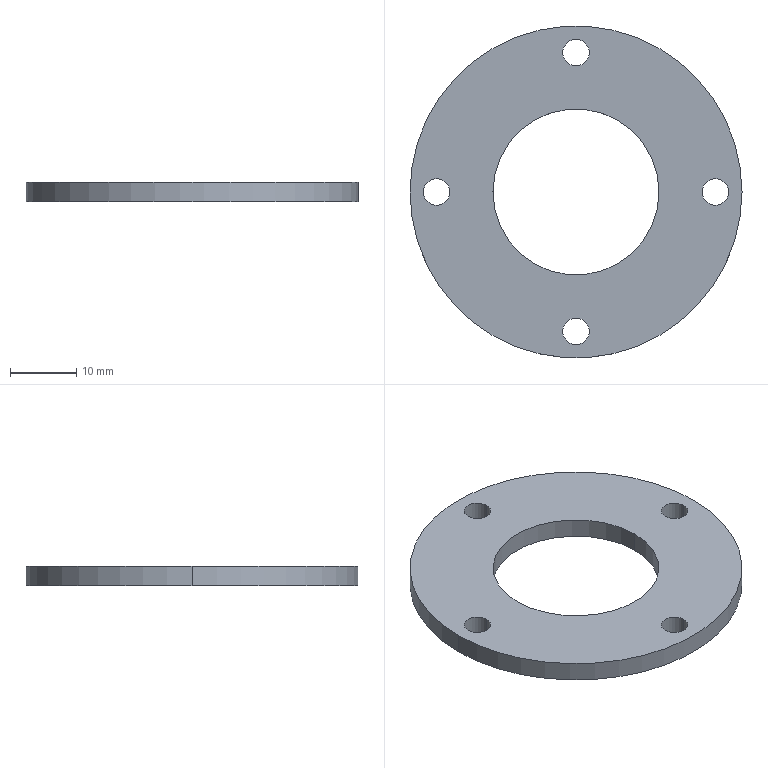Part | SolidWorks | features BaseBody 1 | 1 solid | 14 faces | box 50 x 50 x 3 mm | volume 4267 mm3 | cylinder 12 | plane 2 | commonest cylinder face diameters 4 x8 25 x2 50 x2
STEP:
#1=CARTESIAN_POINT('',(12.5,0.,0.));
#2=VERTEX_POINT('',#1);
#3=CARTESIAN_POINT('',(-12.5,0.,0.));
#4=VERTEX_POINT('',#3);
#5=CARTESIAN_POINT('',(0.,0.,0.));
#6=DIRECTION('',(0.,0.,-1.));
#7=DIRECTION('',(1.,0.,0.));
#8=AXIS2_PLACEMENT_3D('',#5,#6,#7);
#9=CIRCLE('',#8,12.5);
#10=EDGE_CURVE('',#2,#4,#9,.T.);
#11=ORIENTED_EDGE('',*,*,#10,.T.);
#12=CARTESIAN_POINT('',(-12.5,0.,3.));
#13=VERTEX_POINT('',#12);
#14=CARTESIAN_POINT('',(-12.5,0.,0.));
#15=DIRECTION('',(0.,0.,1.));
#16=VECTOR('',#15,1000.);
#17=LINE('',#14,#16);
#18=EDGE_CURVE('',#4,#13,#17,.T.);
#19=ORIENTED_EDGE('',*,*,#18,.T.);
#20=CARTESIAN_POINT('',(12.5,0.,3.));
#21=VERTEX_POINT('',#20);
#22=CARTESIAN_POINT('',(0.,0.,3.));
#23=DIRECTION('',(0.,0.,1.));
#24=DIRECTION('',(1.,0.,0.));
#25=AXIS2_PLACEMENT_3D('',#22,#23,#24);
#26=CIRCLE('',#25,12.5);
#27=EDGE_CURVE('',#13,#21,#26,.T.);
#28=ORIENTED_EDGE('',*,*,#27,.T.);
#29=CARTESIAN_POINT('',(12.5,0.,0.));
#30=DIRECTION('',(0.,0.,1.));
#31=VECTOR('',#30,1000.);
#32=LINE('',#29,#31);
#33=EDGE_CURVE('',#2,#21,#32,.T.);
#34=ORIENTED_EDGE('',*,*,#33,.F.);
#35=EDGE_LOOP('',(#11,#19,#28,#34));
#36=FACE_OUTER_BOUND('',#35,.T.);
#37=CARTESIAN_POINT('',(0.,0.,0.));
#38=DIRECTION('',(0.,0.,1.));
#39=DIRECTION('',(1.,0.,0.));
#40=AXIS2_PLACEMENT_3D('',#37,#38,#39);
#41=CYLINDRICAL_SURFACE('',#40,12.5);
#42=ADVANCED_FACE('',(#36),#41,.F.);
#43=CARTESIAN_POINT('',(2.,21.,0.));
#44=VERTEX_POINT('',#43);
#45=CARTESIAN_POINT('',(-2.,21.,0.));
#46=VERTEX_POINT('',#45);
#47=CARTESIAN_POINT('',(0.,21.,0.));
#48=DIRECTION('',(0.,0.,-1.));
#49=DIRECTION('',(1.,0.,0.));
#50=AXIS2_PLACEMENT_3D('',#47,#48,#49);
#51=CIRCLE('',#50,2.);
#52=EDGE_CURVE('',#44,#46,#51,.T.);
#53=ORIENTED_EDGE('',*,*,#52,.T.);
#54=CARTESIAN_POINT('',(-2.,21.,3.));
#55=VERTEX_POINT('',#54);
#56=CARTESIAN_POINT('',(-2.,21.,0.));
#57=DIRECTION('',(0.,0.,1.));
#58=VECTOR('',#57,1000.);
#59=LINE('',#56,#58);
#60=EDGE_CURVE('',#46,#55,#59,.T.);
#61=ORIENTED_EDGE('',*,*,#60,.T.);
#62=CARTESIAN_POINT('',(2.,21.,3.));
#63=VERTEX_POINT('',#62);
#64=CARTESIAN_POINT('',(0.,21.,3.));
#65=DIRECTION('',(0.,0.,-1.));
#66=DIRECTION('',(1.,0.,0.));
#67=AXIS2_PLACEMENT_3D('',#64,#65,#66);
#68=CIRCLE('',#67,2.);
#69=EDGE_CURVE('',#63,#55,#68,.T.);
#70=ORIENTED_EDGE('',*,*,#69,.F.);
#71=CARTESIAN_POINT('',(2.,21.,0.));
#72=DIRECTION('',(0.,0.,1.));
#73=VECTOR('',#72,1000.);
#74=LINE('',#71,#73);
#75=EDGE_CURVE('',#44,#63,#74,.T.);
#76=ORIENTED_EDGE('',*,*,#75,.F.);
#77=EDGE_LOOP('',(#53,#61,#70,#76));
#78=FACE_OUTER_BOUND('',#77,.T.);
#79=CARTESIAN_POINT('',(0.,21.,0.));
#80=DIRECTION('',(0.,0.,1.));
#81=DIRECTION('',(1.,0.,0.));
#82=AXIS2_PLACEMENT_3D('',#79,#80,#81);
#83=CYLINDRICAL_SURFACE('',#82,2.);
#84=ADVANCED_FACE('',(#78),#83,.F.);
#85=CARTESIAN_POINT('',(23.,0.,0.));
#86=VERTEX_POINT('',#85);
#87=CARTESIAN_POINT('',(19.,0.,0.));
#88=VERTEX_POINT('',#87);
#89=CARTESIAN_POINT('',(21.,0.,0.));
#90=DIRECTION('',(0.,0.,-1.));
#91=DIRECTION('',(1.,0.,0.));
#92=AXIS2_PLACEMENT_3D('',#89,#90,#91);
#93=CIRCLE('',#92,2.);
#94=EDGE_CURVE('',#86,#88,#93,.T.);
#95=ORIENTED_EDGE('',*,*,#94,.T.);
#96=CARTESIAN_POINT('',(19.,0.,3.));
#97=VERTEX_POINT('',#96);
#98=CARTESIAN_POINT('',(19.,0.,0.));
#99=DIRECTION('',(0.,0.,1.));
#100=VECTOR('',#99,1000.);
#101=LINE('',#98,#100);
#102=EDGE_CURVE('',#88,#97,#101,.T.);
#103=ORIENTED_EDGE('',*,*,#102,.T.);
#104=CARTESIAN_POINT('',(23.,0.,3.));
#105=VERTEX_POINT('',#104);
#106=CARTESIAN_POINT('',(21.,0.,3.));
#107=DIRECTION('',(0.,0.,-1.));
#108=DIRECTION('',(1.,0.,0.));
#109=AXIS2_PLACEMENT_3D('',#106,#107,#108);
#110=CIRCLE('',#109,2.);
#111=EDGE_CURVE('',#105,#97,#110,.T.);
#112=ORIENTED_EDGE('',*,*,#111,.F.);
#113=CARTESIAN_POINT('',(23.,0.,0.));
#114=DIRECTION('',(0.,0.,1.));
#115=VECTOR('',#114,1000.);
#116=LINE('',#113,#115);
#117=EDGE_CURVE('',#86,#105,#116,.T.);
#118=ORIENTED_EDGE('',*,*,#117,.F.);
#119=EDGE_LOOP('',(#95,#103,#112,#118));
#120=FACE_OUTER_BOUND('',#119,.T.);
#121=CARTESIAN_POINT('',(21.,0.,0.));
#122=DIRECTION('',(0.,0.,1.));
#123=DIRECTION('',(1.,0.,0.));
#124=AXIS2_PLACEMENT_3D('',#121,#122,#123);
#125=CYLINDRICAL_SURFACE('',#124,2.);
#126=ADVANCED_FACE('',(#120),#125,.F.);
#127=CARTESIAN_POINT('',(2.,-21.,0.));
#128=VERTEX_POINT('',#127);
#129=CARTESIAN_POINT('',(-2.,-21.,0.));
#130=VERTEX_POINT('',#129);
#131=CARTESIAN_POINT('',(0.,-21.,0.));
#132=DIRECTION('',(0.,0.,-1.));
#133=DIRECTION('',(1.,0.,0.));
#134=AXIS2_PLACEMENT_3D('',#131,#132,#133);
#135=CIRCLE('',#134,2.);
#136=EDGE_CURVE('',#128,#130,#135,.T.);
#137=ORIENTED_EDGE('',*,*,#136,.T.);
#138=CARTESIAN_POINT('',(-2.,-21.,3.));
#139=VERTEX_POINT('',#138);
#140=CARTESIAN_POINT('',(-2.,-21.,0.));
#141=DIRECTION('',(0.,0.,1.));
#142=VECTOR('',#141,1000.);
#143=LINE('',#140,#142);
#144=EDGE_CURVE('',#130,#139,#143,.T.);
#145=ORIENTED_EDGE('',*,*,#144,.T.);
#146=CARTESIAN_POINT('',(2.,-21.,3.));
#147=VERTEX_POINT('',#146);
#148=CARTESIAN_POINT('',(0.,-21.,3.));
#149=DIRECTION('',(0.,0.,-1.));
#150=DIRECTION('',(1.,0.,0.));
#151=AXIS2_PLACEMENT_3D('',#148,#149,#150);
#152=CIRCLE('',#151,2.);
#153=EDGE_CURVE('',#147,#139,#152,.T.);
#154=ORIENTED_EDGE('',*,*,#153,.F.);
#155=CARTESIAN_POINT('',(2.,-21.,0.));
#156=DIRECTION('',(0.,0.,1.));
#157=VECTOR('',#156,1000.);
#158=LINE('',#155,#157);
#159=EDGE_CURVE('',#128,#147,#158,.T.);
#160=ORIENTED_EDGE('',*,*,#159,.F.);
#161=EDGE_LOOP('',(#137,#145,#154,#160));
#162=FACE_OUTER_BOUND('',#161,.T.);
#163=CARTESIAN_POINT('',(0.,-21.,0.));
#164=DIRECTION('',(0.,0.,1.));
#165=DIRECTION('',(1.,0.,0.));
#166=AXIS2_PLACEMENT_3D('',#163,#164,#165);
#167=CYLINDRICAL_SURFACE('',#166,2.);
#168=ADVANCED_FACE('',(#162),#167,.F.);
#169=CARTESIAN_POINT('',(-19.,0.,0.));
#170=VERTEX_POINT('',#169);
#171=CARTESIAN_POINT('',(-23.,0.,0.));
#172=VERTEX_POINT('',#171);
#173=CARTESIAN_POINT('',(-21.,0.,0.));
#174=DIRECTION('',(0.,0.,-1.));
#175=DIRECTION('',(1.,0.,0.));
#176=AXIS2_PLACEMENT_3D('',#173,#174,#175);
#177=CIRCLE('',#176,2.);
#178=EDGE_CURVE('',#170,#172,#177,.T.);
#179=ORIENTED_EDGE('',*,*,#178,.T.);
#180=CARTESIAN_POINT('',(-23.,0.,3.));
#181=VERTEX_POINT('',#180);
#182=CARTESIAN_POINT('',(-23.,0.,0.));
#183=DIRECTION('',(0.,0.,1.));
#184=VECTOR('',#183,1000.);
#185=LINE('',#182,#184);
#186=EDGE_CURVE('',#172,#181,#185,.T.);
#187=ORIENTED_EDGE('',*,*,#186,.T.);
#188=CARTESIAN_POINT('',(-19.,0.,3.));
#189=VERTEX_POINT('',#188);
#190=CARTESIAN_POINT('',(-21.,0.,3.));
#191=DIRECTION('',(0.,0.,-1.));
#192=DIRECTION('',(1.,0.,0.));
#193=AXIS2_PLACEMENT_3D('',#190,#191,#192);
#194=CIRCLE('',#193,2.);
#195=EDGE_CURVE('',#189,#181,#194,.T.);
#196=ORIENTED_EDGE('',*,*,#195,.F.);
#197=CARTESIAN_POINT('',(-19.,0.,0.));
#198=DIRECTION('',(0.,0.,1.));
#199=VECTOR('',#198,1000.);
#200=LINE('',#197,#199);
#201=EDGE_CURVE('',#170,#189,#200,.T.);
#202=ORIENTED_EDGE('',*,*,#201,.F.);
#203=EDGE_LOOP('',(#179,#187,#196,#202));
#204=FACE_OUTER_BOUND('',#203,.T.);
#205=CARTESIAN_POINT('',(-21.,0.,0.));
#206=DIRECTION('',(0.,0.,1.));
#207=DIRECTION('',(1.,0.,0.));
#208=AXIS2_PLACEMENT_3D('',#205,#206,#207);
#209=CYLINDRICAL_SURFACE('',#208,2.);
#210=ADVANCED_FACE('',(#204),#209,.F.);
#211=CARTESIAN_POINT('',(25.,0.,3.));
#212=VERTEX_POINT('',#211);
#213=CARTESIAN_POINT('',(-25.,0.,3.));
#214=VERTEX_POINT('',#213);
#215=CARTESIAN_POINT('',(0.,0.,3.));
#216=DIRECTION('',(0.,0.,1.));
#217=DIRECTION('',(-1.,0.,0.));
#218=AXIS2_PLACEMENT_3D('',#215,#216,#217);
#219=CIRCLE('',#218,25.);
#220=EDGE_CURVE('',#212,#214,#219,.T.);
#221=ORIENTED_EDGE('',*,*,#220,.F.);
#222=CARTESIAN_POINT('',(25.,0.,0.));
#223=VERTEX_POINT('',#222);
#224=CARTESIAN_POINT('',(25.,0.,3.));
#225=DIRECTION('',(0.,0.,-1.));
#226=VECTOR('',#225,1000.);
#227=LINE('',#224,#226);
#228=EDGE_CURVE('',#212,#223,#227,.T.);
#229=ORIENTED_EDGE('',*,*,#228,.T.);
#230=CARTESIAN_POINT('',(-25.,0.,0.));
#231=VERTEX_POINT('',#230);
#232=CARTESIAN_POINT('',(0.,0.,0.));
#233=DIRECTION('',(0.,0.,1.));
#234=DIRECTION('',(-1.,0.,0.));
#235=AXIS2_PLACEMENT_3D('',#232,#233,#234);
#236=CIRCLE('',#235,25.);
#237=EDGE_CURVE('',#223,#231,#236,.T.);
#238=ORIENTED_EDGE('',*,*,#237,.T.);
#239=CARTESIAN_POINT('',(-25.,0.,3.));
#240=DIRECTION('',(0.,0.,-1.));
#241=VECTOR('',#240,1000.);
#242=LINE('',#239,#241);
#243=EDGE_CURVE('',#214,#231,#242,.T.);
#244=ORIENTED_EDGE('',*,*,#243,.F.);
#245=EDGE_LOOP('',(#221,#229,#238,#244));
#246=FACE_OUTER_BOUND('',#245,.T.);
#247=CARTESIAN_POINT('',(0.,0.,3.));
#248=DIRECTION('',(0.,0.,-1.));
#249=DIRECTION('',(-1.,0.,0.));
#250=AXIS2_PLACEMENT_3D('',#247,#248,#249);
#251=CYLINDRICAL_SURFACE('',#250,25.);
#252=ADVANCED_FACE('',(#246),#251,.T.);
#253=ORIENTED_EDGE('',*,*,#18,.F.);
#254=CARTESIAN_POINT('',(0.,0.,0.));
#255=DIRECTION('',(0.,0.,-1.));
#256=DIRECTION('',(1.,0.,0.));
#257=AXIS2_PLACEMENT_3D('',#254,#255,#256);
#258=CIRCLE('',#257,12.5);
#259=EDGE_CURVE('',#4,#2,#258,.T.);
#260=ORIENTED_EDGE('',*,*,#259,.T.);
#261=ORIENTED_EDGE('',*,*,#33,.T.);
#262=CARTESIAN_POINT('',(0.,0.,3.));
#263=DIRECTION('',(0.,0.,1.));
#264=DIRECTION('',(1.,0.,0.));
#265=AXIS2_PLACEMENT_3D('',#262,#263,#264);
#266=CIRCLE('',#265,12.5);
#267=EDGE_CURVE('',#21,#13,#266,.T.);
#268=ORIENTED_EDGE('',*,*,#267,.T.);
#269=EDGE_LOOP('',(#253,#260,#261,#268));
#270=FACE_OUTER_BOUND('',#269,.T.);
#271=CARTESIAN_POINT('',(0.,0.,0.));
#272=DIRECTION('',(0.,0.,1.));
#273=DIRECTION('',(1.,0.,0.));
#274=AXIS2_PLACEMENT_3D('',#271,#272,#273);
#275=CYLINDRICAL_SURFACE('',#274,12.5);
#276=ADVANCED_FACE('',(#270),#275,.F.);
#277=ORIENTED_EDGE('',*,*,#69,.T.);
#278=CARTESIAN_POINT('',(0.,21.,3.));
#279=DIRECTION('',(0.,0.,-1.));
#280=DIRECTION('',(1.,0.,0.));
#281=AXIS2_PLACEMENT_3D('',#278,#279,#280);
#282=CIRCLE('',#281,2.);
#283=EDGE_CURVE('',#55,#63,#282,.T.);
#284=ORIENTED_EDGE('',*,*,#283,.T.);
#285=EDGE_LOOP('',(#277,#284));
#286=FACE_BOUND('',#285,.T.);
#287=ORIENTED_EDGE('',*,*,#111,.T.);
#288=CARTESIAN_POINT('',(21.,0.,3.));
#289=DIRECTION('',(0.,0.,-1.));
#290=DIRECTION('',(1.,0.,0.));
#291=AXIS2_PLACEMENT_3D('',#288,#289,#290);
#292=CIRCLE('',#291,2.);
#293=EDGE_CURVE('',#97,#105,#292,.T.);
#294=ORIENTED_EDGE('',*,*,#293,.T.);
#295=EDGE_LOOP('',(#287,#294));
#296=FACE_BOUND('',#295,.T.);
#297=ORIENTED_EDGE('',*,*,#153,.T.);
#298=CARTESIAN_POINT('',(0.,-21.,3.));
#299=DIRECTION('',(0.,0.,-1.));
#300=DIRECTION('',(1.,0.,0.));
#301=AXIS2_PLACEMENT_3D('',#298,#299,#300);
#302=CIRCLE('',#301,2.);
#303=EDGE_CURVE('',#139,#147,#302,.T.);
#304=ORIENTED_EDGE('',*,*,#303,.T.);
#305=EDGE_LOOP('',(#297,#304));
#306=FACE_BOUND('',#305,.T.);
#307=ORIENTED_EDGE('',*,*,#195,.T.);
#308=CARTESIAN_POINT('',(-21.,0.,3.));
#309=DIRECTION('',(0.,0.,-1.));
#310=DIRECTION('',(1.,0.,0.));
#311=AXIS2_PLACEMENT_3D('',#308,#309,#310);
#312=CIRCLE('',#311,2.);
#313=EDGE_CURVE('',#181,#189,#312,.T.);
#314=ORIENTED_EDGE('',*,*,#313,.T.);
#315=EDGE_LOOP('',(#307,#314));
#316=FACE_BOUND('',#315,.T.);
#317=ORIENTED_EDGE('',*,*,#267,.F.);
#318=ORIENTED_EDGE('',*,*,#27,.F.);
#319=EDGE_LOOP('',(#317,#318));
#320=FACE_BOUND('',#319,.T.);
#321=CARTESIAN_POINT('',(0.,0.,3.));
#322=DIRECTION('',(0.,0.,1.));
#323=DIRECTION('',(-1.,0.,0.));
#324=AXIS2_PLACEMENT_3D('',#321,#322,#323);
#325=CIRCLE('',#324,25.);
#326=EDGE_CURVE('',#214,#212,#325,.T.);
#327=ORIENTED_EDGE('',*,*,#326,.T.);
#328=ORIENTED_EDGE('',*,*,#220,.T.);
#329=EDGE_LOOP('',(#327,#328));
#330=FACE_OUTER_BOUND('',#329,.T.);
#331=CARTESIAN_POINT('',(-25.3,-25.3,3.));
#332=DIRECTION('',(0.,0.,1.));
#333=DIRECTION('',(1.,0.,0.));
#334=AXIS2_PLACEMENT_3D('',#331,#332,#333);
#335=PLANE('',#334);
#336=ADVANCED_FACE('',(#286,#296,#306,#316,#320,#330),#335,.T.);
#337=ORIENTED_EDGE('',*,*,#52,.F.);
#338=CARTESIAN_POINT('',(0.,21.,0.));
#339=DIRECTION('',(0.,0.,-1.));
#340=DIRECTION('',(1.,0.,0.));
#341=AXIS2_PLACEMENT_3D('',#338,#339,#340);
#342=CIRCLE('',#341,2.);
#343=EDGE_CURVE('',#46,#44,#342,.T.);
#344=ORIENTED_EDGE('',*,*,#343,.F.);
#345=EDGE_LOOP('',(#337,#344));
#346=FACE_BOUND('',#345,.T.);
#347=ORIENTED_EDGE('',*,*,#94,.F.);
#348=CARTESIAN_POINT('',(21.,0.,0.));
#349=DIRECTION('',(0.,0.,-1.));
#350=DIRECTION('',(1.,0.,0.));
#351=AXIS2_PLACEMENT_3D('',#348,#349,#350);
#352=CIRCLE('',#351,2.);
#353=EDGE_CURVE('',#88,#86,#352,.T.);
#354=ORIENTED_EDGE('',*,*,#353,.F.);
#355=EDGE_LOOP('',(#347,#354));
#356=FACE_BOUND('',#355,.T.);
#357=ORIENTED_EDGE('',*,*,#136,.F.);
#358=CARTESIAN_POINT('',(0.,-21.,0.));
#359=DIRECTION('',(0.,0.,-1.));
#360=DIRECTION('',(1.,0.,0.));
#361=AXIS2_PLACEMENT_3D('',#358,#359,#360);
#362=CIRCLE('',#361,2.);
#363=EDGE_CURVE('',#130,#128,#362,.T.);
#364=ORIENTED_EDGE('',*,*,#363,.F.);
#365=EDGE_LOOP('',(#357,#364));
#366=FACE_BOUND('',#365,.T.);
#367=ORIENTED_EDGE('',*,*,#178,.F.);
#368=CARTESIAN_POINT('',(-21.,0.,0.));
#369=DIRECTION('',(0.,0.,-1.));
#370=DIRECTION('',(1.,0.,0.));
#371=AXIS2_PLACEMENT_3D('',#368,#369,#370);
#372=CIRCLE('',#371,2.);
#373=EDGE_CURVE('',#172,#170,#372,.T.);
#374=ORIENTED_EDGE('',*,*,#373,.F.);
#375=EDGE_LOOP('',(#367,#374));
#376=FACE_BOUND('',#375,.T.);
#377=ORIENTED_EDGE('',*,*,#10,.F.);
#378=ORIENTED_EDGE('',*,*,#259,.F.);
#379=EDGE_LOOP('',(#377,#378));
#380=FACE_BOUND('',#379,.T.);
#381=CARTESIAN_POINT('',(0.,0.,0.));
#382=DIRECTION('',(0.,0.,1.));
#383=DIRECTION('',(-1.,0.,0.));
#384=AXIS2_PLACEMENT_3D('',#381,#382,#383);
#385=CIRCLE('',#384,25.);
#386=EDGE_CURVE('',#231,#223,#385,.T.);
#387=ORIENTED_EDGE('',*,*,#386,.F.);
#388=ORIENTED_EDGE('',*,*,#237,.F.);
#389=EDGE_LOOP('',(#387,#388));
#390=FACE_OUTER_BOUND('',#389,.T.);
#391=CARTESIAN_POINT('',(-25.3,-25.3,0.));
#392=DIRECTION('',(0.,0.,1.));
#393=DIRECTION('',(1.,0.,0.));
#394=AXIS2_PLACEMENT_3D('',#391,#392,#393);
#395=PLANE('',#394);
#396=ADVANCED_FACE('',(#346,#356,#366,#376,#380,#390),#395,.F.);
#397=ORIENTED_EDGE('',*,*,#60,.F.);
#398=ORIENTED_EDGE('',*,*,#343,.T.);
#399=ORIENTED_EDGE('',*,*,#75,.T.);
#400=ORIENTED_EDGE('',*,*,#283,.F.);
#401=EDGE_LOOP('',(#397,#398,#399,#400));
#402=FACE_OUTER_BOUND('',#401,.T.);
#403=CARTESIAN_POINT('',(0.,21.,0.));
#404=DIRECTION('',(0.,0.,1.));
#405=DIRECTION('',(1.,0.,0.));
#406=AXIS2_PLACEMENT_3D('',#403,#404,#405);
#407=CYLINDRICAL_SURFACE('',#406,2.);
#408=ADVANCED_FACE('',(#402),#407,.F.);
#409=ORIENTED_EDGE('',*,*,#102,.F.);
#410=ORIENTED_EDGE('',*,*,#353,.T.);
#411=ORIENTED_EDGE('',*,*,#117,.T.);
#412=ORIENTED_EDGE('',*,*,#293,.F.);
#413=EDGE_LOOP('',(#409,#410,#411,#412));
#414=FACE_OUTER_BOUND('',#413,.T.);
#415=CARTESIAN_POINT('',(21.,0.,0.));
#416=DIRECTION('',(0.,0.,1.));
#417=DIRECTION('',(1.,0.,0.));
#418=AXIS2_PLACEMENT_3D('',#415,#416,#417);
#419=CYLINDRICAL_SURFACE('',#418,2.);
#420=ADVANCED_FACE('',(#414),#419,.F.);
#421=ORIENTED_EDGE('',*,*,#144,.F.);
#422=ORIENTED_EDGE('',*,*,#363,.T.);
#423=ORIENTED_EDGE('',*,*,#159,.T.);
#424=ORIENTED_EDGE('',*,*,#303,.F.);
#425=EDGE_LOOP('',(#421,#422,#423,#424));
#426=FACE_OUTER_BOUND('',#425,.T.);
#427=CARTESIAN_POINT('',(0.,-21.,0.));
#428=DIRECTION('',(0.,0.,1.));
#429=DIRECTION('',(1.,0.,0.));
#430=AXIS2_PLACEMENT_3D('',#427,#428,#429);
#431=CYLINDRICAL_SURFACE('',#430,2.);
#432=ADVANCED_FACE('',(#426),#431,.F.);
#433=ORIENTED_EDGE('',*,*,#186,.F.);
#434=ORIENTED_EDGE('',*,*,#373,.T.);
#435=ORIENTED_EDGE('',*,*,#201,.T.);
#436=ORIENTED_EDGE('',*,*,#313,.F.);
#437=EDGE_LOOP('',(#433,#434,#435,#436));
#438=FACE_OUTER_BOUND('',#437,.T.);
#439=CARTESIAN_POINT('',(-21.,0.,0.));
#440=DIRECTION('',(0.,0.,1.));
#441=DIRECTION('',(1.,0.,0.));
#442=AXIS2_PLACEMENT_3D('',#439,#440,#441);
#443=CYLINDRICAL_SURFACE('',#442,2.);
#444=ADVANCED_FACE('',(#438),#443,.F.);
#445=ORIENTED_EDGE('',*,*,#228,.F.);
#446=ORIENTED_EDGE('',*,*,#326,.F.);
#447=ORIENTED_EDGE('',*,*,#243,.T.);
#448=ORIENTED_EDGE('',*,*,#386,.T.);
#449=EDGE_LOOP('',(#445,#446,#447,#448));
#450=FACE_OUTER_BOUND('',#449,.T.);
#451=CARTESIAN_POINT('',(0.,0.,3.));
#452=DIRECTION('',(0.,0.,-1.));
#453=DIRECTION('',(-1.,0.,0.));
#454=AXIS2_PLACEMENT_3D('',#451,#452,#453);
#455=CYLINDRICAL_SURFACE('',#454,25.);
#456=ADVANCED_FACE('',(#450),#455,.T.);
#457=CLOSED_SHELL('',(#42,#84,#126,#168,#210,#252,#276,#336,#396,#408,#420,#432,#444,#456));
#458=MANIFOLD_SOLID_BREP('',#457);
#459=CARTESIAN_POINT('',(0.,0.,0.));
#460=DIRECTION('',(0.,0.,1.));
#461=DIRECTION('',(1.,0.,0.));
#462=AXIS2_PLACEMENT_3D('',#459,#460,#461);
#463=(LENGTH_UNIT()NAMED_UNIT(*)SI_UNIT(.MILLI.,.METRE.));
#464=UNCERTAINTY_MEASURE_WITH_UNIT(LENGTH_MEASURE(0.00001),#463,'','');
#465=(NAMED_UNIT(*)PLANE_ANGLE_UNIT()SI_UNIT($,.RADIAN.));
#466=(NAMED_UNIT(*)SI_UNIT($,.STERADIAN.)SOLID_ANGLE_UNIT());
#467=(GEOMETRIC_REPRESENTATION_CONTEXT(3)GLOBAL_UNCERTAINTY_ASSIGNED_CONTEXT((#464))GLOBAL_UNIT_ASSIGNED_CONTEXT((#463,#465,#466))REPRESENTATION_CONTEXT('',''));
#468=ADVANCED_BREP_SHAPE_REPRESENTATION('',(#458,#462),#467);